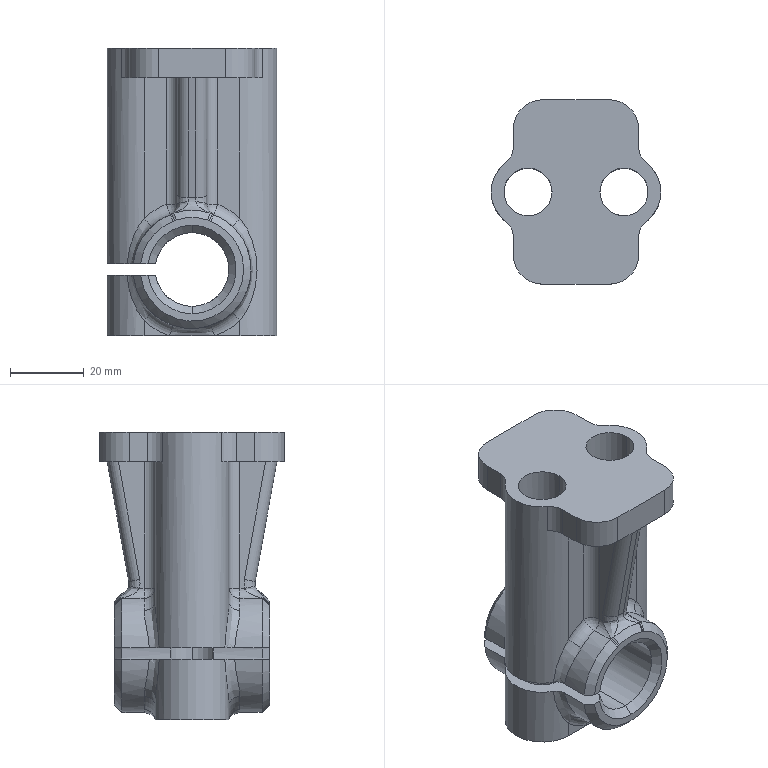Part | SolidWorks | features Fillet 15, ICE 6, Rib 2, Chamfer 1, Extrusion 1 | 1 solid | 117 faces | box 46 x 50 x 78 mm | volume 61833 mm3 | cylinder 37 | plane 28 | spline 25 | cone 15 | torus 8 | sphere 4 | commonest cylinder face diameters 6 x12 20 x7 13 x6 10 x4 16 x4 32 x4